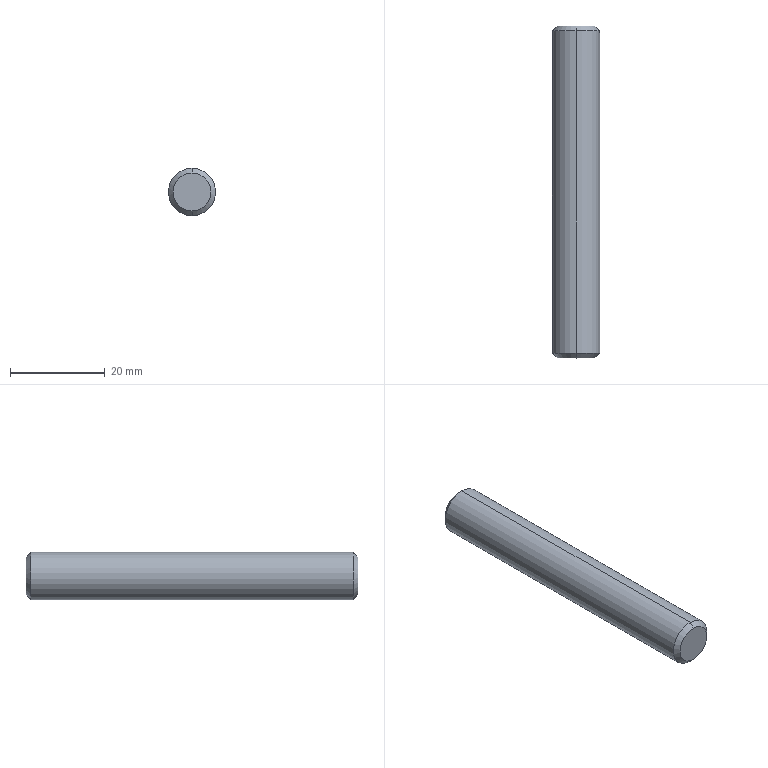Part | STEP file | 1 solid | 8 faces | box 10 x 70 x 10 mm | volume 5468 mm3 | cone 4 | cylinder 2 | plane 2 | commonest cylinder face diameters 10 x2
STEP:
#1=CARTESIAN_POINT('',(0.,0.,0.));
#2=DIRECTION('',(0.,0.,1.));
#3=DIRECTION('',(1.,0.,0.));
#4=AXIS2_PLACEMENT_3D('',#1,#2,#3);
#5=CARTESIAN_POINT('',(0.,70.,4.));
#6=VERTEX_POINT('',#5);
#7=CARTESIAN_POINT('',(0.,70.,-4.));
#8=VERTEX_POINT('',#7);
#9=CARTESIAN_POINT('',(0.,70.,0.));
#10=DIRECTION('',(0.,1.,0.));
#11=DIRECTION('',(0.,0.,1.));
#12=AXIS2_PLACEMENT_3D('',#9,#10,#11);
#13=CIRCLE('',#12,4.);
#14=CARTESIAN_POINT('',(0.,70.,0.));
#15=DIRECTION('',(0.,-1.,0.));
#16=DIRECTION('',(0.,0.,-1.));
#17=AXIS2_PLACEMENT_3D('',#14,#15,#16);
#18=CONICAL_SURFACE('',#17,4.,0.7854);
#19=CARTESIAN_POINT('',(3.142,0.));
#20=DIRECTION('',(-1.,0.));
#21=VECTOR('',#20,1.);
#22=LINE('',#19,#21);
#23=(GEOMETRIC_REPRESENTATION_CONTEXT(2)PARAMETRIC_REPRESENTATION_CONTEXT()REPRESENTATION_CONTEXT('',''));
#24=DEFINITIONAL_REPRESENTATION('',(#22),#23);
#25=PCURVE('',#18,#24);
#26=CARTESIAN_POINT('',(0.,70.,0.));
#27=DIRECTION('',(0.,1.,0.));
#28=DIRECTION('',(0.,0.,1.));
#29=AXIS2_PLACEMENT_3D('',#26,#27,#28);
#30=PLANE('',#29);
#31=CARTESIAN_POINT('',(0.,0.));
#32=DIRECTION('',(1.,0.));
#33=AXIS2_PLACEMENT_2D('',#31,#32);
#34=CIRCLE('',#33,4.);
#35=(GEOMETRIC_REPRESENTATION_CONTEXT(2)PARAMETRIC_REPRESENTATION_CONTEXT()REPRESENTATION_CONTEXT('',''));
#36=DEFINITIONAL_REPRESENTATION('',(#34),#35);
#37=PCURVE('',#30,#36);
#38=SURFACE_CURVE('',#13,(#25,#37),.PCURVE_S1.);
#39=EDGE_CURVE('',#6,#8,#38,.T.);
#40=ORIENTED_EDGE('',*,*,#39,.F.);
#41=CARTESIAN_POINT('',(0.,69.,5.));
#42=VERTEX_POINT('',#41);
#43=CARTESIAN_POINT('',(0.,70.,4.));
#44=DIRECTION('',(0.,-0.7071,0.7071));
#45=VECTOR('',#44,1.);
#46=LINE('',#43,#45);
#47=CARTESIAN_POINT('',(3.142,0.));
#48=DIRECTION('',(0.,1.));
#49=VECTOR('',#48,1.);
#50=LINE('',#47,#49);
#51=(GEOMETRIC_REPRESENTATION_CONTEXT(2)PARAMETRIC_REPRESENTATION_CONTEXT()REPRESENTATION_CONTEXT('',''));
#52=DEFINITIONAL_REPRESENTATION('',(#50),#51);
#53=PCURVE('',#18,#52);
#54=CARTESIAN_POINT('',(0.,70.,0.));
#55=DIRECTION('',(0.,-1.,0.));
#56=DIRECTION('',(0.,0.,-1.));
#57=AXIS2_PLACEMENT_3D('',#54,#55,#56);
#58=CONICAL_SURFACE('',#57,4.,0.7854);
#59=CARTESIAN_POINT('',(3.142,0.));
#60=DIRECTION('',(0.,1.));
#61=VECTOR('',#60,1.);
#62=LINE('',#59,#61);
#63=(GEOMETRIC_REPRESENTATION_CONTEXT(2)PARAMETRIC_REPRESENTATION_CONTEXT()REPRESENTATION_CONTEXT('',''));
#64=DEFINITIONAL_REPRESENTATION('',(#62),#63);
#65=PCURVE('',#58,#64);
#66=SURFACE_CURVE('',#46,(#53,#65),.PCURVE_S1.);
#67=EDGE_CURVE('',#6,#42,#66,.T.);
#68=ORIENTED_EDGE('',*,*,#67,.T.);
#69=CARTESIAN_POINT('',(0.,69.,-5.));
#70=VERTEX_POINT('',#69);
#71=CARTESIAN_POINT('',(0.,69.,0.));
#72=DIRECTION('',(0.,-1.,0.));
#73=DIRECTION('',(0.,0.,1.));
#74=AXIS2_PLACEMENT_3D('',#71,#72,#73);
#75=CIRCLE('',#74,5.);
#76=CARTESIAN_POINT('',(-3.142,1.));
#77=DIRECTION('',(1.,0.));
#78=VECTOR('',#77,1.);
#79=LINE('',#76,#78);
#80=(GEOMETRIC_REPRESENTATION_CONTEXT(2)PARAMETRIC_REPRESENTATION_CONTEXT()REPRESENTATION_CONTEXT('',''));
#81=DEFINITIONAL_REPRESENTATION('',(#79),#80);
#82=PCURVE('',#18,#81);
#83=CARTESIAN_POINT('',(0.,70.,0.));
#84=DIRECTION('',(0.,-1.,0.));
#85=DIRECTION('',(0.,0.,-1.));
#86=AXIS2_PLACEMENT_3D('',#83,#84,#85);
#87=CYLINDRICAL_SURFACE('',#86,5.);
#88=CARTESIAN_POINT('',(-3.142,1.));
#89=DIRECTION('',(1.,0.));
#90=VECTOR('',#89,1.);
#91=LINE('',#88,#90);
#92=(GEOMETRIC_REPRESENTATION_CONTEXT(2)PARAMETRIC_REPRESENTATION_CONTEXT()REPRESENTATION_CONTEXT('',''));
#93=DEFINITIONAL_REPRESENTATION('',(#91),#92);
#94=PCURVE('',#87,#93);
#95=SURFACE_CURVE('',#75,(#82,#94),.PCURVE_S1.);
#96=EDGE_CURVE('',#70,#42,#95,.T.);
#97=ORIENTED_EDGE('',*,*,#96,.F.);
#98=CARTESIAN_POINT('',(0.,70.,-4.));
#99=DIRECTION('',(0.,-0.7071,-0.7071));
#100=VECTOR('',#99,1.);
#101=LINE('',#98,#100);
#102=CARTESIAN_POINT('',(0.,0.));
#103=DIRECTION('',(0.,1.));
#104=VECTOR('',#103,1.);
#105=LINE('',#102,#104);
#106=(GEOMETRIC_REPRESENTATION_CONTEXT(2)PARAMETRIC_REPRESENTATION_CONTEXT()REPRESENTATION_CONTEXT('',''));
#107=DEFINITIONAL_REPRESENTATION('',(#105),#106);
#108=PCURVE('',#18,#107);
#109=CARTESIAN_POINT('',(6.283,0.));
#110=DIRECTION('',(0.,1.));
#111=VECTOR('',#110,1.);
#112=LINE('',#109,#111);
#113=(GEOMETRIC_REPRESENTATION_CONTEXT(2)PARAMETRIC_REPRESENTATION_CONTEXT()REPRESENTATION_CONTEXT('',''));
#114=DEFINITIONAL_REPRESENTATION('',(#112),#113);
#115=PCURVE('',#58,#114);
#116=SURFACE_CURVE('',#101,(#108,#115),.PCURVE_S1.);
#117=EDGE_CURVE('',#8,#70,#116,.T.);
#118=ORIENTED_EDGE('',*,*,#117,.F.);
#119=EDGE_LOOP('',(#40,#68,#97,#118));
#120=FACE_BOUND('',#119,.T.);
#121=ADVANCED_FACE('',(#120),#18,.T.);
#122=CARTESIAN_POINT('',(0.,0.,-4.));
#123=VERTEX_POINT('',#122);
#124=CARTESIAN_POINT('',(0.,0.,4.));
#125=VERTEX_POINT('',#124);
#126=CARTESIAN_POINT('',(0.,0.,0.));
#127=DIRECTION('',(0.,-1.,0.));
#128=DIRECTION('',(0.,0.,1.));
#129=AXIS2_PLACEMENT_3D('',#126,#127,#128);
#130=CIRCLE('',#129,4.);
#131=CARTESIAN_POINT('',(0.,1.,0.));
#132=DIRECTION('',(0.,1.,0.));
#133=DIRECTION('',(0.,0.,1.));
#134=AXIS2_PLACEMENT_3D('',#131,#132,#133);
#135=CONICAL_SURFACE('',#134,5.,0.7854);
#136=CARTESIAN_POINT('',(6.283,-1.));
#137=DIRECTION('',(-1.,0.));
#138=VECTOR('',#137,1.);
#139=LINE('',#136,#138);
#140=(GEOMETRIC_REPRESENTATION_CONTEXT(2)PARAMETRIC_REPRESENTATION_CONTEXT()REPRESENTATION_CONTEXT('',''));
#141=DEFINITIONAL_REPRESENTATION('',(#139),#140);
#142=PCURVE('',#135,#141);
#143=CARTESIAN_POINT('',(0.,0.,0.));
#144=DIRECTION('',(0.,1.,0.));
#145=DIRECTION('',(0.,0.,1.));
#146=AXIS2_PLACEMENT_3D('',#143,#144,#145);
#147=PLANE('',#146);
#148=CARTESIAN_POINT('',(4.,0.));
#149=CARTESIAN_POINT('',(4.,-6.928));
#150=CARTESIAN_POINT('',(-2.,-3.464));
#151=CARTESIAN_POINT('',(-8.,0.));
#152=CARTESIAN_POINT('',(-2.,3.464));
#153=CARTESIAN_POINT('',(4.,6.928));
#154=CARTESIAN_POINT('',(4.,0.));
#155=(BOUNDED_CURVE()B_SPLINE_CURVE(2,(#148,#149,#150,#151,#152,#153,#154),.UNSPECIFIED.,.T.,.F.)B_SPLINE_CURVE_WITH_KNOTS((1,2,2,2,2,1),(-2.094,0.,2.094,4.189,6.283,8.378),.UNSPECIFIED.)CURVE()GEOMETRIC_REPRESENTATION_ITEM()RATIONAL_B_SPLINE_CURVE((1.,0.5,1.,0.5,1.,0.5,1.))REPRESENTATION_ITEM(''));
#156=(GEOMETRIC_REPRESENTATION_CONTEXT(2)PARAMETRIC_REPRESENTATION_CONTEXT()REPRESENTATION_CONTEXT('',''));
#157=DEFINITIONAL_REPRESENTATION('',(#155),#156);
#158=PCURVE('',#147,#157);
#159=SURFACE_CURVE('',#130,(#142,#158),.PCURVE_S1.);
#160=EDGE_CURVE('',#123,#125,#159,.T.);
#161=ORIENTED_EDGE('',*,*,#160,.F.);
#162=CARTESIAN_POINT('',(0.,1.,-5.));
#163=VERTEX_POINT('',#162);
#164=CARTESIAN_POINT('',(0.,1.,-5.));
#165=DIRECTION('',(0.,0.7071,-0.7071));
#166=VECTOR('',#165,1.);
#167=LINE('',#164,#166);
#168=CARTESIAN_POINT('',(3.142,0.));
#169=DIRECTION('',(0.,1.));
#170=VECTOR('',#169,1.);
#171=LINE('',#168,#170);
#172=(GEOMETRIC_REPRESENTATION_CONTEXT(2)PARAMETRIC_REPRESENTATION_CONTEXT()REPRESENTATION_CONTEXT('',''));
#173=DEFINITIONAL_REPRESENTATION('',(#171),#172);
#174=PCURVE('',#135,#173);
#175=CARTESIAN_POINT('',(0.,1.,0.));
#176=DIRECTION('',(0.,1.,0.));
#177=DIRECTION('',(0.,0.,1.));
#178=AXIS2_PLACEMENT_3D('',#175,#176,#177);
#179=CONICAL_SURFACE('',#178,5.,0.7854);
#180=CARTESIAN_POINT('',(3.142,0.));
#181=DIRECTION('',(0.,1.));
#182=VECTOR('',#181,1.);
#183=LINE('',#180,#182);
#184=(GEOMETRIC_REPRESENTATION_CONTEXT(2)PARAMETRIC_REPRESENTATION_CONTEXT()REPRESENTATION_CONTEXT('',''));
#185=DEFINITIONAL_REPRESENTATION('',(#183),#184);
#186=PCURVE('',#179,#185);
#187=SURFACE_CURVE('',#167,(#174,#186),.PCURVE_S1.);
#188=EDGE_CURVE('',#123,#163,#187,.T.);
#189=ORIENTED_EDGE('',*,*,#188,.T.);
#190=CARTESIAN_POINT('',(0.,1.,5.));
#191=VERTEX_POINT('',#190);
#192=CARTESIAN_POINT('',(0.,1.,0.));
#193=DIRECTION('',(0.,1.,0.));
#194=DIRECTION('',(0.,0.,1.));
#195=AXIS2_PLACEMENT_3D('',#192,#193,#194);
#196=CIRCLE('',#195,5.);
#197=CARTESIAN_POINT('',(0.,0.));
#198=DIRECTION('',(1.,0.));
#199=VECTOR('',#198,1.);
#200=LINE('',#197,#199);
#201=(GEOMETRIC_REPRESENTATION_CONTEXT(2)PARAMETRIC_REPRESENTATION_CONTEXT()REPRESENTATION_CONTEXT('',''));
#202=DEFINITIONAL_REPRESENTATION('',(#200),#201);
#203=PCURVE('',#135,#202);
#204=CARTESIAN_POINT('',(3.142,69.));
#205=DIRECTION('',(-1.,0.));
#206=VECTOR('',#205,1.);
#207=LINE('',#204,#206);
#208=(GEOMETRIC_REPRESENTATION_CONTEXT(2)PARAMETRIC_REPRESENTATION_CONTEXT()REPRESENTATION_CONTEXT('',''));
#209=DEFINITIONAL_REPRESENTATION('',(#207),#208);
#210=PCURVE('',#87,#209);
#211=SURFACE_CURVE('',#196,(#203,#210),.PCURVE_S1.);
#212=EDGE_CURVE('',#191,#163,#211,.T.);
#213=ORIENTED_EDGE('',*,*,#212,.F.);
#214=CARTESIAN_POINT('',(0.,1.,5.));
#215=DIRECTION('',(0.,0.7071,0.7071));
#216=VECTOR('',#215,1.);
#217=LINE('',#214,#216);
#218=CARTESIAN_POINT('',(0.,0.));
#219=DIRECTION('',(0.,1.));
#220=VECTOR('',#219,1.);
#221=LINE('',#218,#220);
#222=(GEOMETRIC_REPRESENTATION_CONTEXT(2)PARAMETRIC_REPRESENTATION_CONTEXT()REPRESENTATION_CONTEXT('',''));
#223=DEFINITIONAL_REPRESENTATION('',(#221),#222);
#224=PCURVE('',#135,#223);
#225=CARTESIAN_POINT('',(6.283,0.));
#226=DIRECTION('',(0.,1.));
#227=VECTOR('',#226,1.);
#228=LINE('',#225,#227);
#229=(GEOMETRIC_REPRESENTATION_CONTEXT(2)PARAMETRIC_REPRESENTATION_CONTEXT()REPRESENTATION_CONTEXT('',''));
#230=DEFINITIONAL_REPRESENTATION('',(#228),#229);
#231=PCURVE('',#179,#230);
#232=SURFACE_CURVE('',#217,(#224,#231),.PCURVE_S1.);
#233=EDGE_CURVE('',#125,#191,#232,.T.);
#234=ORIENTED_EDGE('',*,*,#233,.F.);
#235=EDGE_LOOP('',(#161,#189,#213,#234));
#236=FACE_BOUND('',#235,.T.);
#237=ADVANCED_FACE('',(#236),#135,.T.);
#238=ORIENTED_EDGE('',*,*,#96,.T.);
#239=CARTESIAN_POINT('',(0.,70.,5.));
#240=DIRECTION('',(0.,-1.,0.));
#241=VECTOR('',#240,1.);
#242=LINE('',#239,#241);
#243=CARTESIAN_POINT('',(3.142,0.));
#244=DIRECTION('',(0.,1.));
#245=VECTOR('',#244,1.);
#246=LINE('',#243,#245);
#247=(GEOMETRIC_REPRESENTATION_CONTEXT(2)PARAMETRIC_REPRESENTATION_CONTEXT()REPRESENTATION_CONTEXT('',''));
#248=DEFINITIONAL_REPRESENTATION('',(#246),#247);
#249=PCURVE('',#87,#248);
#250=CARTESIAN_POINT('',(0.,70.,0.));
#251=DIRECTION('',(0.,-1.,0.));
#252=DIRECTION('',(0.,0.,-1.));
#253=AXIS2_PLACEMENT_3D('',#250,#251,#252);
#254=CYLINDRICAL_SURFACE('',#253,5.);
#255=CARTESIAN_POINT('',(3.142,0.));
#256=DIRECTION('',(0.,1.));
#257=VECTOR('',#256,1.);
#258=LINE('',#255,#257);
#259=(GEOMETRIC_REPRESENTATION_CONTEXT(2)PARAMETRIC_REPRESENTATION_CONTEXT()REPRESENTATION_CONTEXT('',''));
#260=DEFINITIONAL_REPRESENTATION('',(#258),#259);
#261=PCURVE('',#254,#260);
#262=SURFACE_CURVE('',#242,(#249,#261),.PCURVE_S1.);
#263=EDGE_CURVE('',#42,#191,#262,.T.);
#264=ORIENTED_EDGE('',*,*,#263,.T.);
#265=ORIENTED_EDGE('',*,*,#212,.T.);
#266=CARTESIAN_POINT('',(0.,70.,-5.));
#267=DIRECTION('',(0.,-1.,0.));
#268=VECTOR('',#267,1.);
#269=LINE('',#266,#268);
#270=CARTESIAN_POINT('',(0.,0.));
#271=DIRECTION('',(0.,1.));
#272=VECTOR('',#271,1.);
#273=LINE('',#270,#272);
#274=(GEOMETRIC_REPRESENTATION_CONTEXT(2)PARAMETRIC_REPRESENTATION_CONTEXT()REPRESENTATION_CONTEXT('',''));
#275=DEFINITIONAL_REPRESENTATION('',(#273),#274);
#276=PCURVE('',#87,#275);
#277=CARTESIAN_POINT('',(6.283,0.));
#278=DIRECTION('',(0.,1.));
#279=VECTOR('',#278,1.);
#280=LINE('',#277,#279);
#281=(GEOMETRIC_REPRESENTATION_CONTEXT(2)PARAMETRIC_REPRESENTATION_CONTEXT()REPRESENTATION_CONTEXT('',''));
#282=DEFINITIONAL_REPRESENTATION('',(#280),#281);
#283=PCURVE('',#254,#282);
#284=SURFACE_CURVE('',#269,(#276,#283),.PCURVE_S1.);
#285=EDGE_CURVE('',#70,#163,#284,.T.);
#286=ORIENTED_EDGE('',*,*,#285,.F.);
#287=EDGE_LOOP('',(#238,#264,#265,#286));
#288=FACE_BOUND('',#287,.T.);
#289=ADVANCED_FACE('',(#288),#87,.T.);
#290=ORIENTED_EDGE('',*,*,#263,.F.);
#291=CARTESIAN_POINT('',(0.,69.,0.));
#292=DIRECTION('',(0.,-1.,0.));
#293=DIRECTION('',(0.,0.,1.));
#294=AXIS2_PLACEMENT_3D('',#291,#292,#293);
#295=CIRCLE('',#294,5.);
#296=CARTESIAN_POINT('',(3.142,1.));
#297=DIRECTION('',(1.,0.));
#298=VECTOR('',#297,1.);
#299=LINE('',#296,#298);
#300=(GEOMETRIC_REPRESENTATION_CONTEXT(2)PARAMETRIC_REPRESENTATION_CONTEXT()REPRESENTATION_CONTEXT('',''));
#301=DEFINITIONAL_REPRESENTATION('',(#299),#300);
#302=PCURVE('',#254,#301);
#303=CARTESIAN_POINT('',(3.142,1.));
#304=DIRECTION('',(1.,0.));
#305=VECTOR('',#304,1.);
#306=LINE('',#303,#305);
#307=(GEOMETRIC_REPRESENTATION_CONTEXT(2)PARAMETRIC_REPRESENTATION_CONTEXT()REPRESENTATION_CONTEXT('',''));
#308=DEFINITIONAL_REPRESENTATION('',(#306),#307);
#309=PCURVE('',#58,#308);
#310=SURFACE_CURVE('',#295,(#302,#309),.PCURVE_S1.);
#311=EDGE_CURVE('',#42,#70,#310,.T.);
#312=ORIENTED_EDGE('',*,*,#311,.T.);
#313=ORIENTED_EDGE('',*,*,#285,.T.);
#314=CARTESIAN_POINT('',(0.,1.,0.));
#315=DIRECTION('',(0.,1.,0.));
#316=DIRECTION('',(0.,0.,1.));
#317=AXIS2_PLACEMENT_3D('',#314,#315,#316);
#318=CIRCLE('',#317,5.);
#319=CARTESIAN_POINT('',(9.425,69.));
#320=DIRECTION('',(-1.,0.));
#321=VECTOR('',#320,1.);
#322=LINE('',#319,#321);
#323=(GEOMETRIC_REPRESENTATION_CONTEXT(2)PARAMETRIC_REPRESENTATION_CONTEXT()REPRESENTATION_CONTEXT('',''));
#324=DEFINITIONAL_REPRESENTATION('',(#322),#323);
#325=PCURVE('',#254,#324);
#326=CARTESIAN_POINT('',(0.,0.));
#327=DIRECTION('',(1.,0.));
#328=VECTOR('',#327,1.);
#329=LINE('',#326,#328);
#330=(GEOMETRIC_REPRESENTATION_CONTEXT(2)PARAMETRIC_REPRESENTATION_CONTEXT()REPRESENTATION_CONTEXT('',''));
#331=DEFINITIONAL_REPRESENTATION('',(#329),#330);
#332=PCURVE('',#179,#331);
#333=SURFACE_CURVE('',#318,(#325,#332),.PCURVE_S1.);
#334=EDGE_CURVE('',#163,#191,#333,.T.);
#335=ORIENTED_EDGE('',*,*,#334,.T.);
#336=EDGE_LOOP('',(#290,#312,#313,#335));
#337=FACE_BOUND('',#336,.T.);
#338=ADVANCED_FACE('',(#337),#254,.T.);
#339=CARTESIAN_POINT('',(0.,70.,0.));
#340=DIRECTION('',(0.,1.,0.));
#341=DIRECTION('',(0.,0.,1.));
#342=AXIS2_PLACEMENT_3D('',#339,#340,#341);
#343=CIRCLE('',#342,4.);
#344=CARTESIAN_POINT('',(0.,0.));
#345=DIRECTION('',(1.,0.));
#346=AXIS2_PLACEMENT_2D('',#344,#345);
#347=CIRCLE('',#346,4.);
#348=(GEOMETRIC_REPRESENTATION_CONTEXT(2)PARAMETRIC_REPRESENTATION_CONTEXT()REPRESENTATION_CONTEXT('',''));
#349=DEFINITIONAL_REPRESENTATION('',(#347),#348);
#350=PCURVE('',#30,#349);
#351=CARTESIAN_POINT('',(9.425,0.));
#352=DIRECTION('',(-1.,0.));
#353=VECTOR('',#352,1.);
#354=LINE('',#351,#353);
#355=(GEOMETRIC_REPRESENTATION_CONTEXT(2)PARAMETRIC_REPRESENTATION_CONTEXT()REPRESENTATION_CONTEXT('',''));
#356=DEFINITIONAL_REPRESENTATION('',(#354),#355);
#357=PCURVE('',#58,#356);
#358=SURFACE_CURVE('',#343,(#350,#357),.PCURVE_S1.);
#359=EDGE_CURVE('',#8,#6,#358,.T.);
#360=ORIENTED_EDGE('',*,*,#359,.T.);
#361=ORIENTED_EDGE('',*,*,#39,.T.);
#362=EDGE_LOOP('',(#360,#361));
#363=FACE_BOUND('',#362,.T.);
#364=ADVANCED_FACE('',(#363),#30,.T.);
#365=CARTESIAN_POINT('',(0.,0.,0.));
#366=DIRECTION('',(0.,-1.,0.));
#367=DIRECTION('',(0.,0.,1.));
#368=AXIS2_PLACEMENT_3D('',#365,#366,#367);
#369=CIRCLE('',#368,4.);
#370=CARTESIAN_POINT('',(4.,0.));
#371=CARTESIAN_POINT('',(4.,-6.928));
#372=CARTESIAN_POINT('',(-2.,-3.464));
#373=CARTESIAN_POINT('',(-8.,0.));
#374=CARTESIAN_POINT('',(-2.,3.464));
#375=CARTESIAN_POINT('',(4.,6.928));
#376=CARTESIAN_POINT('',(4.,0.));
#377=(BOUNDED_CURVE()B_SPLINE_CURVE(2,(#370,#371,#372,#373,#374,#375,#376),.UNSPECIFIED.,.T.,.F.)B_SPLINE_CURVE_WITH_KNOTS((1,2,2,2,2,1),(-2.094,0.,2.094,4.189,6.283,8.378),.UNSPECIFIED.)CURVE()GEOMETRIC_REPRESENTATION_ITEM()RATIONAL_B_SPLINE_CURVE((1.,0.5,1.,0.5,1.,0.5,1.))REPRESENTATION_ITEM(''));
#378=(GEOMETRIC_REPRESENTATION_CONTEXT(2)PARAMETRIC_REPRESENTATION_CONTEXT()REPRESENTATION_CONTEXT('',''));
#379=DEFINITIONAL_REPRESENTATION('',(#377),#378);
#380=PCURVE('',#147,#379);
#381=CARTESIAN_POINT('',(6.283,-1.));
#382=DIRECTION('',(-1.,0.));
#383=VECTOR('',#382,1.);
#384=LINE('',#381,#383);
#385=(GEOMETRIC_REPRESENTATION_CONTEXT(2)PARAMETRIC_REPRESENTATION_CONTEXT()REPRESENTATION_CONTEXT('',''));
#386=DEFINITIONAL_REPRESENTATION('',(#384),#385);
#387=PCURVE('',#179,#386);
#388=SURFACE_CURVE('',#369,(#380,#387),.PCURVE_S1.);
#389=EDGE_CURVE('',#125,#123,#388,.T.);
#390=ORIENTED_EDGE('',*,*,#389,.T.);
#391=ORIENTED_EDGE('',*,*,#160,.T.);
#392=EDGE_LOOP('',(#390,#391));
#393=FACE_BOUND('',#392,.T.);
#394=ADVANCED_FACE('',(#393),#147,.F.);
#395=ORIENTED_EDGE('',*,*,#188,.F.);
#396=ORIENTED_EDGE('',*,*,#389,.F.);
#397=ORIENTED_EDGE('',*,*,#233,.T.);
#398=ORIENTED_EDGE('',*,*,#334,.F.);
#399=EDGE_LOOP('',(#395,#396,#397,#398));
#400=FACE_BOUND('',#399,.T.);
#401=ADVANCED_FACE('',(#400),#179,.T.);
#402=ORIENTED_EDGE('',*,*,#67,.F.);
#403=ORIENTED_EDGE('',*,*,#359,.F.);
#404=ORIENTED_EDGE('',*,*,#117,.T.);
#405=ORIENTED_EDGE('',*,*,#311,.F.);
#406=EDGE_LOOP('',(#402,#403,#404,#405));
#407=FACE_BOUND('',#406,.T.);
#408=ADVANCED_FACE('',(#407),#58,.T.);
#409=CLOSED_SHELL('',(#121,#237,#289,#338,#364,#394,#401,#408));
#410=MANIFOLD_SOLID_BREP('',#409);
#411=(LENGTH_UNIT()NAMED_UNIT(*)SI_UNIT(.MILLI.,.METRE.));
#412=UNCERTAINTY_MEASURE_WITH_UNIT(LENGTH_MEASURE(0.0000001),#411,'','');
#413=(NAMED_UNIT(*)PLANE_ANGLE_UNIT()SI_UNIT($,.RADIAN.));
#414=(NAMED_UNIT(*)SI_UNIT($,.STERADIAN.)SOLID_ANGLE_UNIT());
#415=(GEOMETRIC_REPRESENTATION_CONTEXT(3)GLOBAL_UNCERTAINTY_ASSIGNED_CONTEXT((#412))GLOBAL_UNIT_ASSIGNED_CONTEXT((#411,#413,#414))REPRESENTATION_CONTEXT('',''));
#416=ADVANCED_BREP_SHAPE_REPRESENTATION('',(#4,#410),#415);